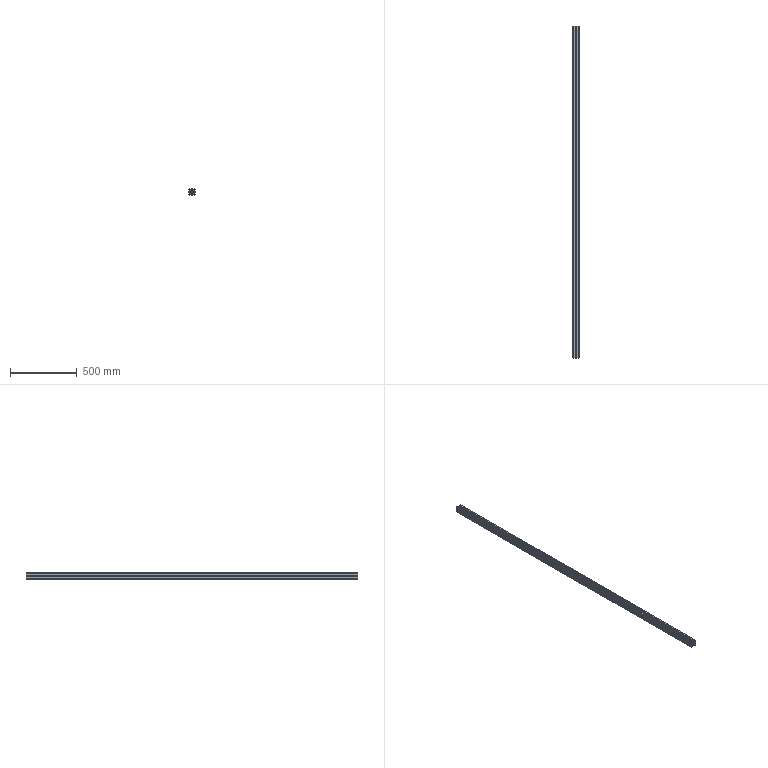Part | STEP file | 1 solid | 135 faces | box 45 x 2481 x 45 mm | volume 1717571 mm3 | plane 118 | cylinder 17 | commonest cylinder face diameters 10 x9 3 x4 5 x4